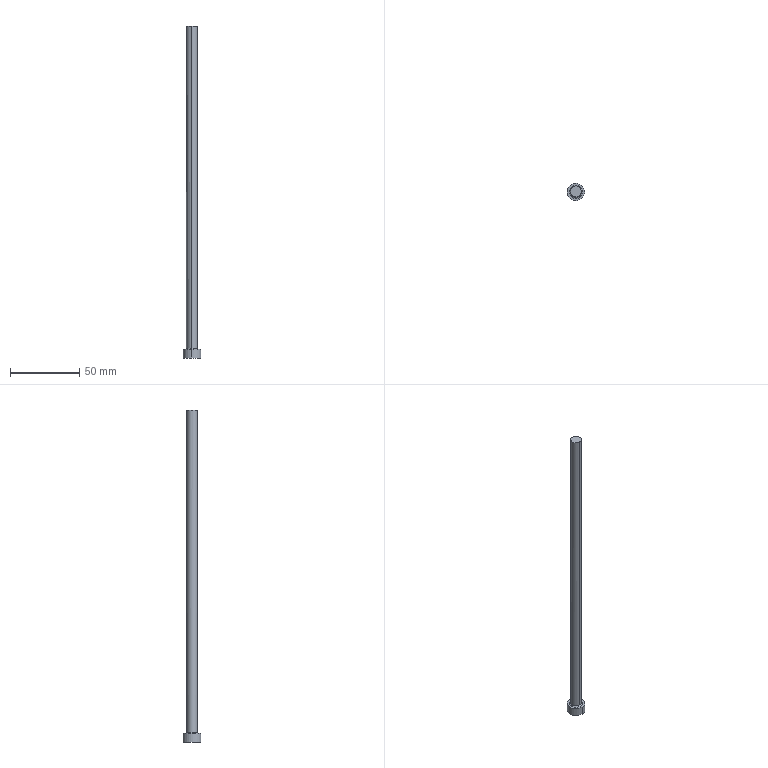Part | STEP file | 4-20.sldasm-Part-229 | 1 solid | 11 faces | box 12.7 x 12.7 x 240.5 mm | volume 12432 mm3 | cylinder 6 | plane 3 | torus 2 | commonest cylinder face diameters 7.95 x3 12.7 x3
STEP:
#1=CARTESIAN_POINT('',(6.35,0.,-105.));
#2=VERTEX_POINT('',#1);
#3=CARTESIAN_POINT('',(0.,-6.35,-105.));
#4=VERTEX_POINT('',#3);
#5=CARTESIAN_POINT('',(0.,0.,-105.));
#6=DIRECTION('',(0.,0.,-1.));
#7=DIRECTION('',(0.,1.,0.));
#8=AXIS2_PLACEMENT_3D('',#5,#6,#7);
#9=CIRCLE('',#8,6.35);
#10=EDGE_CURVE('',#2,#4,#9,.T.);
#11=ORIENTED_EDGE('',*,*,#10,.F.);
#12=CARTESIAN_POINT('',(6.35,0.,-98.65));
#13=VERTEX_POINT('',#12);
#14=CARTESIAN_POINT('',(6.35,0.,-101.825));
#15=DIRECTION('',(0.,0.,1.));
#16=VECTOR('',#15,1000.);
#17=LINE('',#14,#16);
#18=EDGE_CURVE('',#2,#13,#17,.T.);
#19=ORIENTED_EDGE('',*,*,#18,.T.);
#20=CARTESIAN_POINT('',(0.,-6.35,-98.65));
#21=VERTEX_POINT('',#20);
#22=CARTESIAN_POINT('',(0.,0.,-98.65));
#23=DIRECTION('',(0.,0.,-1.));
#24=DIRECTION('',(0.,1.,0.));
#25=AXIS2_PLACEMENT_3D('',#22,#23,#24);
#26=CIRCLE('',#25,6.35);
#27=EDGE_CURVE('',#13,#21,#26,.T.);
#28=ORIENTED_EDGE('',*,*,#27,.T.);
#29=CARTESIAN_POINT('',(0.,-6.35,-101.825));
#30=DIRECTION('',(0.,0.,1.));
#31=VECTOR('',#30,1000.);
#32=LINE('',#29,#31);
#33=EDGE_CURVE('',#4,#21,#32,.T.);
#34=ORIENTED_EDGE('',*,*,#33,.F.);
#35=EDGE_LOOP('',(#11,#19,#28,#34));
#36=FACE_OUTER_BOUND('',#35,.T.);
#37=CARTESIAN_POINT('',(0.,0.,-101.825));
#38=DIRECTION('',(0.,0.,1.));
#39=DIRECTION('',(1.,0.,0.));
#40=AXIS2_PLACEMENT_3D('',#37,#38,#39);
#41=CYLINDRICAL_SURFACE('',#40,6.35);
#42=ADVANCED_FACE('',(#36),#41,.T.);
#43=CARTESIAN_POINT('',(3.975,0.,-97.856));
#44=VERTEX_POINT('',#43);
#45=CARTESIAN_POINT('',(0.,-3.975,-97.856));
#46=VERTEX_POINT('',#45);
#47=CARTESIAN_POINT('',(0.,0.,-97.856));
#48=DIRECTION('',(0.,0.,-1.));
#49=DIRECTION('',(0.,1.,0.));
#50=AXIS2_PLACEMENT_3D('',#47,#48,#49);
#51=CIRCLE('',#50,3.975);
#52=EDGE_CURVE('',#44,#46,#51,.T.);
#53=ORIENTED_EDGE('',*,*,#52,.F.);
#54=CARTESIAN_POINT('',(3.975,0.,135.5));
#55=VERTEX_POINT('',#54);
#56=CARTESIAN_POINT('',(3.975,0.,-25.228));
#57=DIRECTION('',(0.,0.,1.));
#58=VECTOR('',#57,1000.);
#59=LINE('',#56,#58);
#60=EDGE_CURVE('',#44,#55,#59,.T.);
#61=ORIENTED_EDGE('',*,*,#60,.T.);
#62=CARTESIAN_POINT('',(0.,-3.975,135.5));
#63=VERTEX_POINT('',#62);
#64=CARTESIAN_POINT('',(0.,0.,135.5));
#65=DIRECTION('',(0.,0.,-1.));
#66=DIRECTION('',(1.,0.,0.));
#67=AXIS2_PLACEMENT_3D('',#64,#65,#66);
#68=CIRCLE('',#67,3.975);
#69=EDGE_CURVE('',#55,#63,#68,.T.);
#70=ORIENTED_EDGE('',*,*,#69,.T.);
#71=CARTESIAN_POINT('',(0.,-3.975,-25.228));
#72=DIRECTION('',(0.,0.,1.));
#73=VECTOR('',#72,1000.);
#74=LINE('',#71,#73);
#75=EDGE_CURVE('',#46,#63,#74,.T.);
#76=ORIENTED_EDGE('',*,*,#75,.F.);
#77=EDGE_LOOP('',(#53,#61,#70,#76));
#78=FACE_OUTER_BOUND('',#77,.T.);
#79=CARTESIAN_POINT('',(0.,0.,-25.228));
#80=DIRECTION('',(0.,0.,1.));
#81=DIRECTION('',(1.,0.,0.));
#82=AXIS2_PLACEMENT_3D('',#79,#80,#81);
#83=CYLINDRICAL_SURFACE('',#82,3.975);
#84=ADVANCED_FACE('',(#78),#83,.T.);
#85=ORIENTED_EDGE('',*,*,#60,.F.);
#86=CARTESIAN_POINT('',(0.,3.975,-97.856));
#87=VERTEX_POINT('',#86);
#88=CARTESIAN_POINT('',(0.,0.,-97.856));
#89=DIRECTION('',(0.,0.,-1.));
#90=DIRECTION('',(0.,1.,0.));
#91=AXIS2_PLACEMENT_3D('',#88,#89,#90);
#92=CIRCLE('',#91,3.975);
#93=EDGE_CURVE('',#87,#44,#92,.T.);
#94=ORIENTED_EDGE('',*,*,#93,.F.);
#95=CARTESIAN_POINT('',(0.,3.975,135.5));
#96=VERTEX_POINT('',#95);
#97=CARTESIAN_POINT('',(0.,3.975,-25.228));
#98=DIRECTION('',(0.,0.,-1.));
#99=VECTOR('',#98,1000.);
#100=LINE('',#97,#99);
#101=EDGE_CURVE('',#96,#87,#100,.T.);
#102=ORIENTED_EDGE('',*,*,#101,.F.);
#103=CARTESIAN_POINT('',(0.,0.,135.5));
#104=DIRECTION('',(0.,0.,-1.));
#105=DIRECTION('',(1.,0.,0.));
#106=AXIS2_PLACEMENT_3D('',#103,#104,#105);
#107=CIRCLE('',#106,3.975);
#108=EDGE_CURVE('',#96,#55,#107,.T.);
#109=ORIENTED_EDGE('',*,*,#108,.T.);
#110=EDGE_LOOP('',(#85,#94,#102,#109));
#111=FACE_OUTER_BOUND('',#110,.T.);
#112=CARTESIAN_POINT('',(0.,0.,-25.228));
#113=DIRECTION('',(0.,0.,1.));
#114=DIRECTION('',(1.,0.,0.));
#115=AXIS2_PLACEMENT_3D('',#112,#113,#114);
#116=CYLINDRICAL_SURFACE('',#115,3.975);
#117=ADVANCED_FACE('',(#111),#116,.T.);
#118=ORIENTED_EDGE('',*,*,#75,.T.);
#119=CARTESIAN_POINT('',(0.,0.,135.5));
#120=DIRECTION('',(0.,0.,-1.));
#121=DIRECTION('',(1.,0.,0.));
#122=AXIS2_PLACEMENT_3D('',#119,#120,#121);
#123=CIRCLE('',#122,3.975);
#124=EDGE_CURVE('',#63,#96,#123,.T.);
#125=ORIENTED_EDGE('',*,*,#124,.T.);
#126=ORIENTED_EDGE('',*,*,#101,.T.);
#127=CARTESIAN_POINT('',(-3.975,0.,-97.856));
#128=VERTEX_POINT('',#127);
#129=CARTESIAN_POINT('',(0.,0.,-97.856));
#130=DIRECTION('',(0.,0.,-1.));
#131=DIRECTION('',(0.,1.,0.));
#132=AXIS2_PLACEMENT_3D('',#129,#130,#131);
#133=CIRCLE('',#132,3.975);
#134=EDGE_CURVE('',#128,#87,#133,.T.);
#135=ORIENTED_EDGE('',*,*,#134,.F.);
#136=CARTESIAN_POINT('',(0.,0.,-97.856));
#137=DIRECTION('',(0.,0.,-1.));
#138=DIRECTION('',(0.,1.,0.));
#139=AXIS2_PLACEMENT_3D('',#136,#137,#138);
#140=CIRCLE('',#139,3.975);
#141=EDGE_CURVE('',#46,#128,#140,.T.);
#142=ORIENTED_EDGE('',*,*,#141,.F.);
#143=EDGE_LOOP('',(#118,#125,#126,#135,#142));
#144=FACE_OUTER_BOUND('',#143,.T.);
#145=CARTESIAN_POINT('',(0.,0.,-25.228));
#146=DIRECTION('',(0.,0.,1.));
#147=DIRECTION('',(1.,0.,0.));
#148=AXIS2_PLACEMENT_3D('',#145,#146,#147);
#149=CYLINDRICAL_SURFACE('',#148,3.975);
#150=ADVANCED_FACE('',(#144),#149,.T.);
#151=ORIENTED_EDGE('',*,*,#18,.F.);
#152=CARTESIAN_POINT('',(0.,6.35,-105.));
#153=VERTEX_POINT('',#152);
#154=CARTESIAN_POINT('',(0.,0.,-105.));
#155=DIRECTION('',(0.,0.,-1.));
#156=DIRECTION('',(0.,1.,0.));
#157=AXIS2_PLACEMENT_3D('',#154,#155,#156);
#158=CIRCLE('',#157,6.35);
#159=EDGE_CURVE('',#153,#2,#158,.T.);
#160=ORIENTED_EDGE('',*,*,#159,.F.);
#161=CARTESIAN_POINT('',(0.,6.35,-98.65));
#162=VERTEX_POINT('',#161);
#163=CARTESIAN_POINT('',(0.,6.35,-101.825));
#164=DIRECTION('',(0.,0.,-1.));
#165=VECTOR('',#164,1000.);
#166=LINE('',#163,#165);
#167=EDGE_CURVE('',#162,#153,#166,.T.);
#168=ORIENTED_EDGE('',*,*,#167,.F.);
#169=CARTESIAN_POINT('',(0.,0.,-98.65));
#170=DIRECTION('',(0.,0.,-1.));
#171=DIRECTION('',(0.,1.,0.));
#172=AXIS2_PLACEMENT_3D('',#169,#170,#171);
#173=CIRCLE('',#172,6.35);
#174=EDGE_CURVE('',#162,#13,#173,.T.);
#175=ORIENTED_EDGE('',*,*,#174,.T.);
#176=EDGE_LOOP('',(#151,#160,#168,#175));
#177=FACE_OUTER_BOUND('',#176,.T.);
#178=CARTESIAN_POINT('',(0.,0.,-101.825));
#179=DIRECTION('',(0.,0.,1.));
#180=DIRECTION('',(1.,0.,0.));
#181=AXIS2_PLACEMENT_3D('',#178,#179,#180);
#182=CYLINDRICAL_SURFACE('',#181,6.35);
#183=ADVANCED_FACE('',(#177),#182,.T.);
#184=CARTESIAN_POINT('',(4.769,0.,-98.65));
#185=VERTEX_POINT('',#184);
#186=CARTESIAN_POINT('',(4.769,0.,-97.856));
#187=DIRECTION('',(0.,-1.,0.));
#188=DIRECTION('',(1.,0.,0.));
#189=AXIS2_PLACEMENT_3D('',#186,#187,#188);
#190=CIRCLE('',#189,0.7938);
#191=EDGE_CURVE('',#44,#185,#190,.T.);
#192=ORIENTED_EDGE('',*,*,#191,.F.);
#193=ORIENTED_EDGE('',*,*,#52,.T.);
#194=ORIENTED_EDGE('',*,*,#141,.T.);
#195=CARTESIAN_POINT('',(-4.769,0.,-98.65));
#196=VERTEX_POINT('',#195);
#197=CARTESIAN_POINT('',(-4.769,0.,-97.856));
#198=DIRECTION('',(0.,-1.,0.));
#199=DIRECTION('',(-1.,0.,0.));
#200=AXIS2_PLACEMENT_3D('',#197,#198,#199);
#201=CIRCLE('',#200,0.7938);
#202=EDGE_CURVE('',#196,#128,#201,.T.);
#203=ORIENTED_EDGE('',*,*,#202,.F.);
#204=CARTESIAN_POINT('',(0.,0.,-98.65));
#205=DIRECTION('',(0.,0.,-1.));
#206=DIRECTION('',(0.,1.,0.));
#207=AXIS2_PLACEMENT_3D('',#204,#205,#206);
#208=CIRCLE('',#207,4.769);
#209=EDGE_CURVE('',#185,#196,#208,.T.);
#210=ORIENTED_EDGE('',*,*,#209,.F.);
#211=EDGE_LOOP('',(#192,#193,#194,#203,#210));
#212=FACE_OUTER_BOUND('',#211,.T.);
#213=CARTESIAN_POINT('',(0.,0.,-97.856));
#214=DIRECTION('',(0.,0.,-1.));
#215=DIRECTION('',(-1.,0.,0.));
#216=AXIS2_PLACEMENT_3D('',#213,#214,#215);
#217=TOROIDAL_SURFACE('',#216,4.769,0.7937);
#218=ADVANCED_FACE('',(#212),#217,.F.);
#219=ORIENTED_EDGE('',*,*,#191,.T.);
#220=CARTESIAN_POINT('',(0.,0.,-98.65));
#221=DIRECTION('',(0.,0.,-1.));
#222=DIRECTION('',(0.,1.,0.));
#223=AXIS2_PLACEMENT_3D('',#220,#221,#222);
#224=CIRCLE('',#223,4.769);
#225=EDGE_CURVE('',#196,#185,#224,.T.);
#226=ORIENTED_EDGE('',*,*,#225,.F.);
#227=ORIENTED_EDGE('',*,*,#202,.T.);
#228=ORIENTED_EDGE('',*,*,#134,.T.);
#229=ORIENTED_EDGE('',*,*,#93,.T.);
#230=EDGE_LOOP('',(#219,#226,#227,#228,#229));
#231=FACE_OUTER_BOUND('',#230,.T.);
#232=CARTESIAN_POINT('',(0.,0.,-97.856));
#233=DIRECTION('',(0.,0.,-1.));
#234=DIRECTION('',(-1.,0.,0.));
#235=AXIS2_PLACEMENT_3D('',#232,#233,#234);
#236=TOROIDAL_SURFACE('',#235,4.769,0.7937);
#237=ADVANCED_FACE('',(#231),#236,.F.);
#238=ORIENTED_EDGE('',*,*,#174,.F.);
#239=CARTESIAN_POINT('',(0.,0.,-98.65));
#240=DIRECTION('',(0.,0.,-1.));
#241=DIRECTION('',(0.,1.,0.));
#242=AXIS2_PLACEMENT_3D('',#239,#240,#241);
#243=CIRCLE('',#242,6.35);
#244=EDGE_CURVE('',#21,#162,#243,.T.);
#245=ORIENTED_EDGE('',*,*,#244,.F.);
#246=ORIENTED_EDGE('',*,*,#27,.F.);
#247=EDGE_LOOP('',(#238,#245,#246));
#248=FACE_OUTER_BOUND('',#247,.T.);
#249=ORIENTED_EDGE('',*,*,#225,.T.);
#250=ORIENTED_EDGE('',*,*,#209,.T.);
#251=EDGE_LOOP('',(#249,#250));
#252=FACE_BOUND('',#251,.T.);
#253=CARTESIAN_POINT('',(0.,5.559,-98.65));
#254=DIRECTION('',(0.,0.,1.));
#255=DIRECTION('',(0.,1.,0.));
#256=AXIS2_PLACEMENT_3D('',#253,#254,#255);
#257=PLANE('',#256);
#258=ADVANCED_FACE('',(#248,#252),#257,.T.);
#259=ORIENTED_EDGE('',*,*,#167,.T.);
#260=CARTESIAN_POINT('',(0.,0.,-105.));
#261=DIRECTION('',(0.,0.,-1.));
#262=DIRECTION('',(0.,1.,0.));
#263=AXIS2_PLACEMENT_3D('',#260,#261,#262);
#264=CIRCLE('',#263,6.35);
#265=EDGE_CURVE('',#4,#153,#264,.T.);
#266=ORIENTED_EDGE('',*,*,#265,.F.);
#267=ORIENTED_EDGE('',*,*,#33,.T.);
#268=ORIENTED_EDGE('',*,*,#244,.T.);
#269=EDGE_LOOP('',(#259,#266,#267,#268));
#270=FACE_OUTER_BOUND('',#269,.T.);
#271=CARTESIAN_POINT('',(0.,0.,-101.825));
#272=DIRECTION('',(0.,0.,1.));
#273=DIRECTION('',(1.,0.,0.));
#274=AXIS2_PLACEMENT_3D('',#271,#272,#273);
#275=CYLINDRICAL_SURFACE('',#274,6.35);
#276=ADVANCED_FACE('',(#270),#275,.T.);
#277=ORIENTED_EDGE('',*,*,#159,.T.);
#278=ORIENTED_EDGE('',*,*,#10,.T.);
#279=ORIENTED_EDGE('',*,*,#265,.T.);
#280=EDGE_LOOP('',(#277,#278,#279));
#281=FACE_OUTER_BOUND('',#280,.T.);
#282=CARTESIAN_POINT('',(0.,3.175,-105.));
#283=DIRECTION('',(0.,0.,-1.));
#284=DIRECTION('',(-1.,0.,0.));
#285=AXIS2_PLACEMENT_3D('',#282,#283,#284);
#286=PLANE('',#285);
#287=ADVANCED_FACE('',(#281),#286,.T.);
#288=ORIENTED_EDGE('',*,*,#108,.F.);
#289=ORIENTED_EDGE('',*,*,#124,.F.);
#290=ORIENTED_EDGE('',*,*,#69,.F.);
#291=EDGE_LOOP('',(#288,#289,#290));
#292=FACE_OUTER_BOUND('',#291,.T.);
#293=CARTESIAN_POINT('',(0.,0.,135.5));
#294=DIRECTION('',(0.,0.,1.));
#295=DIRECTION('',(1.,0.,0.));
#296=AXIS2_PLACEMENT_3D('',#293,#294,#295);
#297=PLANE('',#296);
#298=ADVANCED_FACE('',(#292),#297,.T.);
#299=CLOSED_SHELL('',(#42,#84,#117,#150,#183,#218,#237,#258,#276,#287,#298));
#300=MANIFOLD_SOLID_BREP('',#299);
#301=CARTESIAN_POINT('',(0.,0.,0.));
#302=DIRECTION('',(0.,0.,1.));
#303=DIRECTION('',(1.,0.,0.));
#304=AXIS2_PLACEMENT_3D('',#301,#302,#303);
#305=(LENGTH_UNIT()NAMED_UNIT(*)SI_UNIT(.MILLI.,.METRE.));
#306=UNCERTAINTY_MEASURE_WITH_UNIT(LENGTH_MEASURE(0.00001),#305,'','');
#307=(NAMED_UNIT(*)PLANE_ANGLE_UNIT()SI_UNIT($,.RADIAN.));
#308=(NAMED_UNIT(*)SI_UNIT($,.STERADIAN.)SOLID_ANGLE_UNIT());
#309=(GEOMETRIC_REPRESENTATION_CONTEXT(3)GLOBAL_UNCERTAINTY_ASSIGNED_CONTEXT((#306))GLOBAL_UNIT_ASSIGNED_CONTEXT((#305,#307,#308))REPRESENTATION_CONTEXT('',''));
#310=ADVANCED_BREP_SHAPE_REPRESENTATION('',(#300,#304),#309);